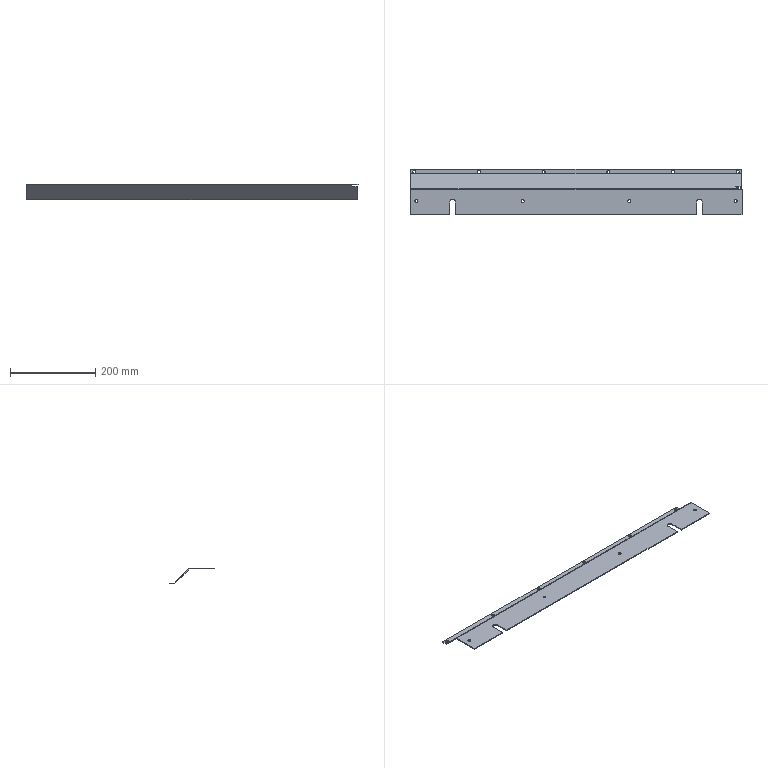Part | STEP file | Wheel Fixing Plate | 1 solid | 51 faces | box 780 x 107 x 37 mm | volume 186121 mm3 | cylinder 26 | plane 25 | commonest cylinder face diameters 7 x20 0.2 x2 4.2 x2 13 x2